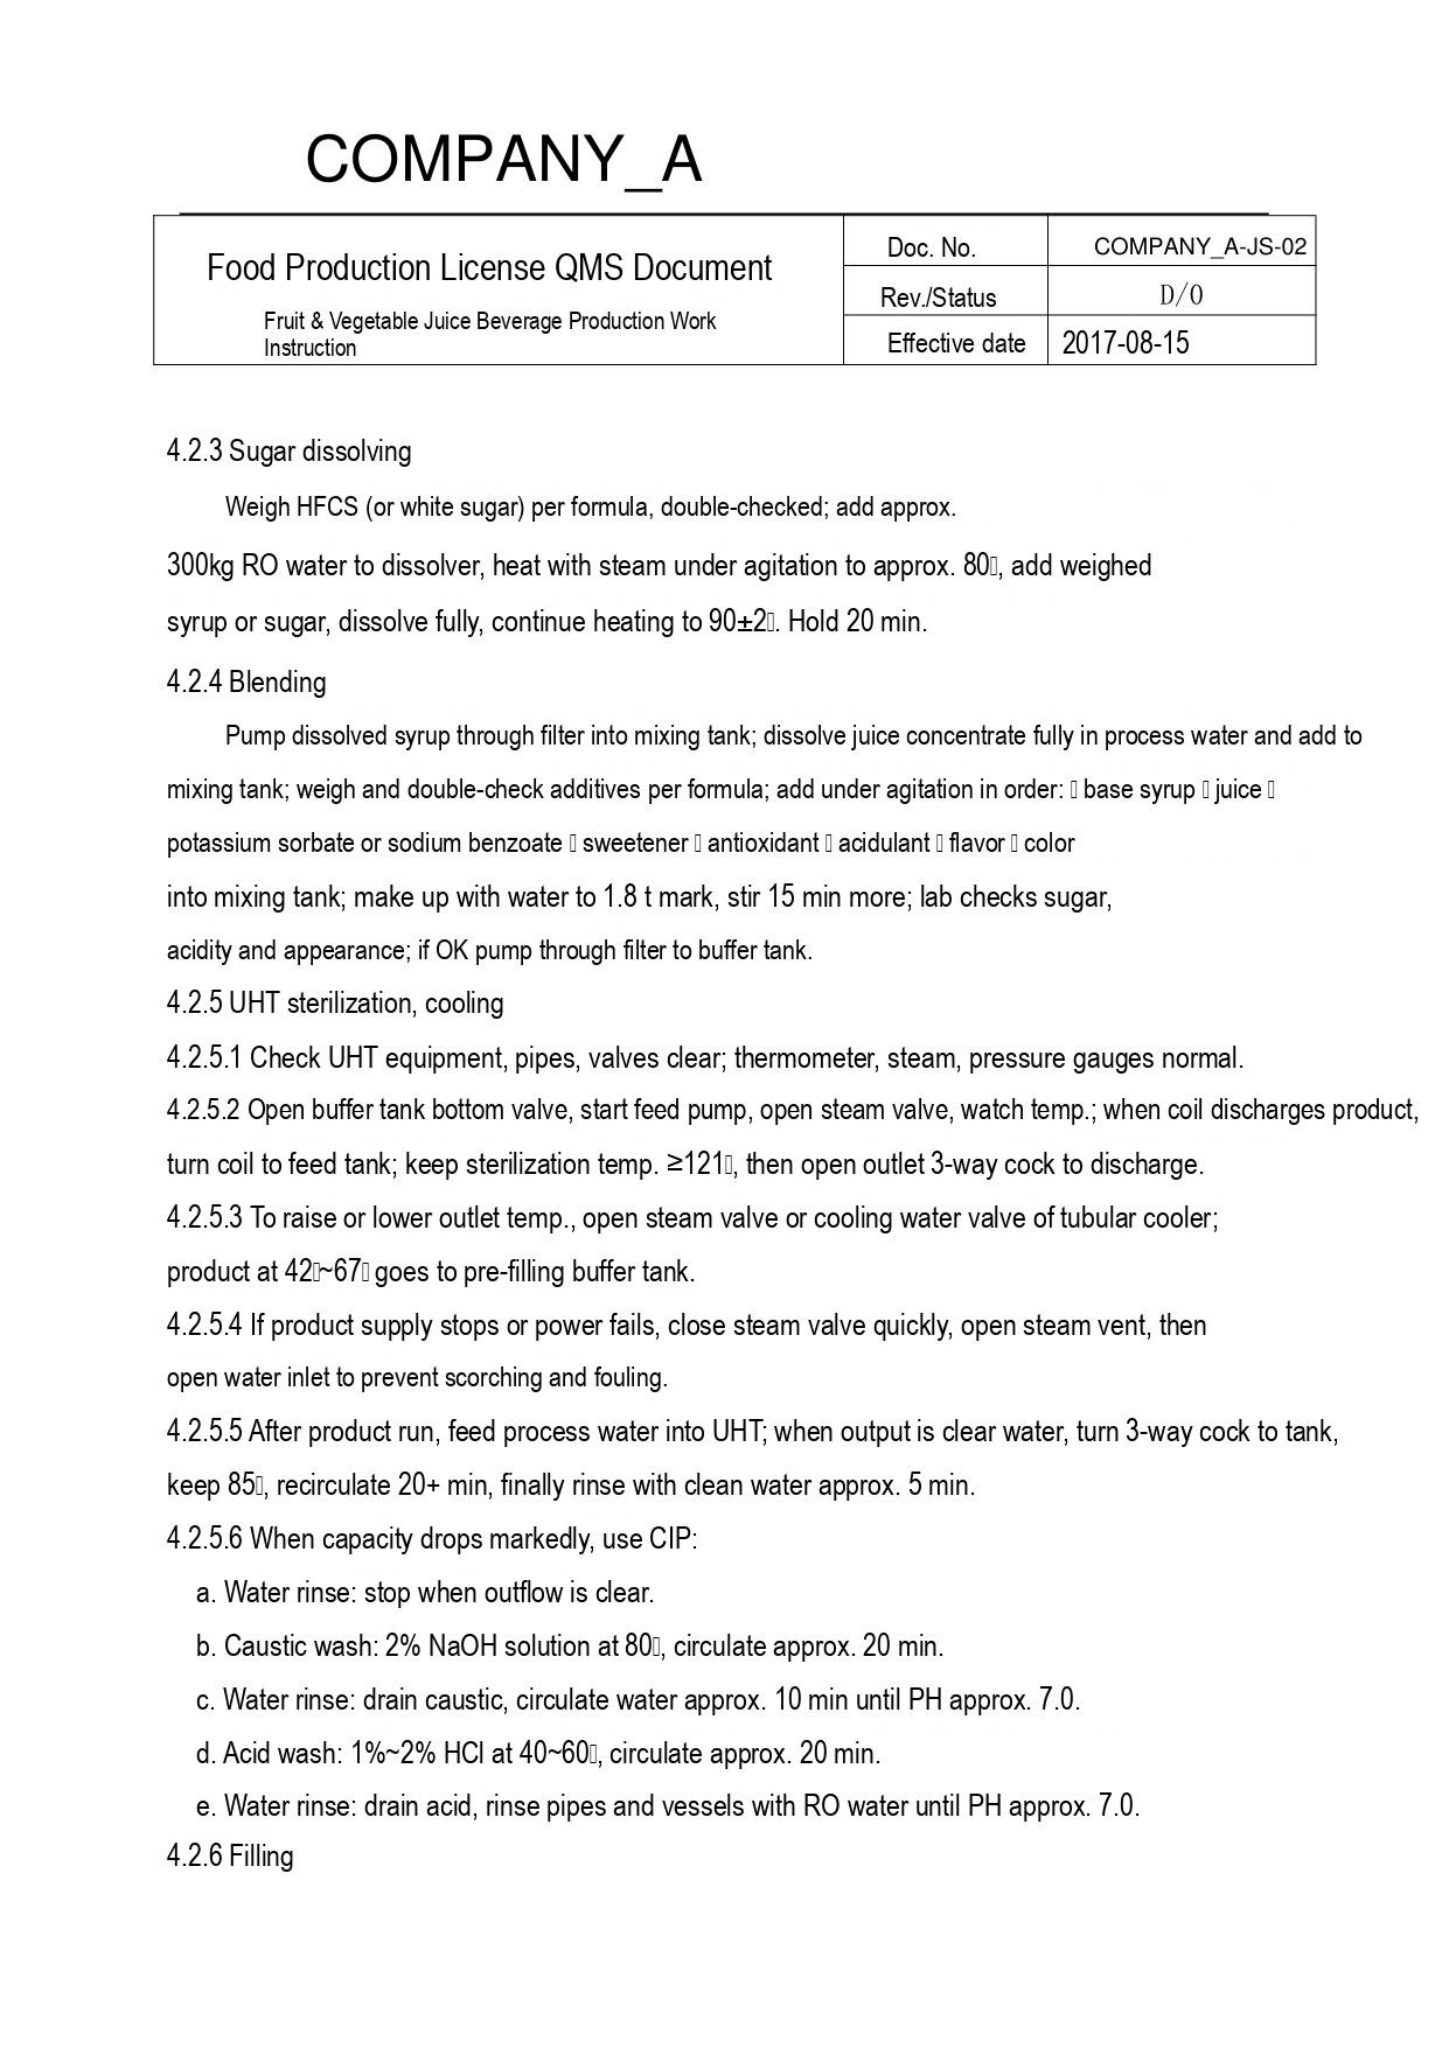COMPANY_A

| Food Production License QMS Document<br>Fruit & Vegetable Juice Beverage Production Work Instruction | Doc. No. | COMPANY_A-JS-02 |
|---|---|---|
| | Rev./Status | D/0 |
| | Effective date | 2017-08-15 |

4.2.3 Sugar dissolving

Weigh HFCS (or white sugar) per formula, double-checked; add approx. 300kg RO water to dissolver, heat with steam under agitation to approx. 80□, add weighed syrup or sugar, dissolve fully, continue heating to 90±2□. Hold 20 min.

4.2.4 Blending

Pump dissolved syrup through filter into mixing tank; dissolve juice concentrate fully in process water and add to mixing tank; weigh and double-check additives per formula; add under agitation in order: □ base syrup □ juice □ potassium sorbate or sodium benzoate □ sweetener □ antioxidant □ acidulant □ flavor □ color into mixing tank; make up with water to 1.8 t mark, stir 15 min more; lab checks sugar, acidity and appearance; if OK pump through filter to buffer tank.

4.2.5 UHT sterilization, cooling

4.2.5.1 Check UHT equipment, pipes, valves clear; thermometer, steam, pressure gauges normal.

4.2.5.2 Open buffer tank bottom valve, start feed pump, open steam valve, watch temp.; when coil discharges product, turn coil to feed tank; keep sterilization temp. ≥121□, then open outlet 3-way cock to discharge.

4.2.5.3 To raise or lower outlet temp., open steam valve or cooling water valve of tubular cooler; product at 42□~67□ goes to pre-filling buffer tank.

4.2.5.4 If product supply stops or power fails, close steam valve quickly, open steam vent, then open water inlet to prevent scorching and fouling.

4.2.5.5 After product run, feed process water into UHT; when output is clear water, turn 3-way cock to tank, keep 85□, recirculate 20+ min, finally rinse with clean water approx. 5 min.

4.2.5.6 When capacity drops markedly, use CIP:

a. Water rinse: stop when outflow is clear.

b. Caustic wash: 2% NaOH solution at 80□, circulate approx. 20 min.

c. Water rinse: drain caustic, circulate water approx. 10 min until PH approx. 7.0.

d. Acid wash: 1%~2% HCl at 40~60□, circulate approx. 20 min.

e. Water rinse: drain acid, rinse pipes and vessels with RO water until PH approx. 7.0.

4.2.6 Filling
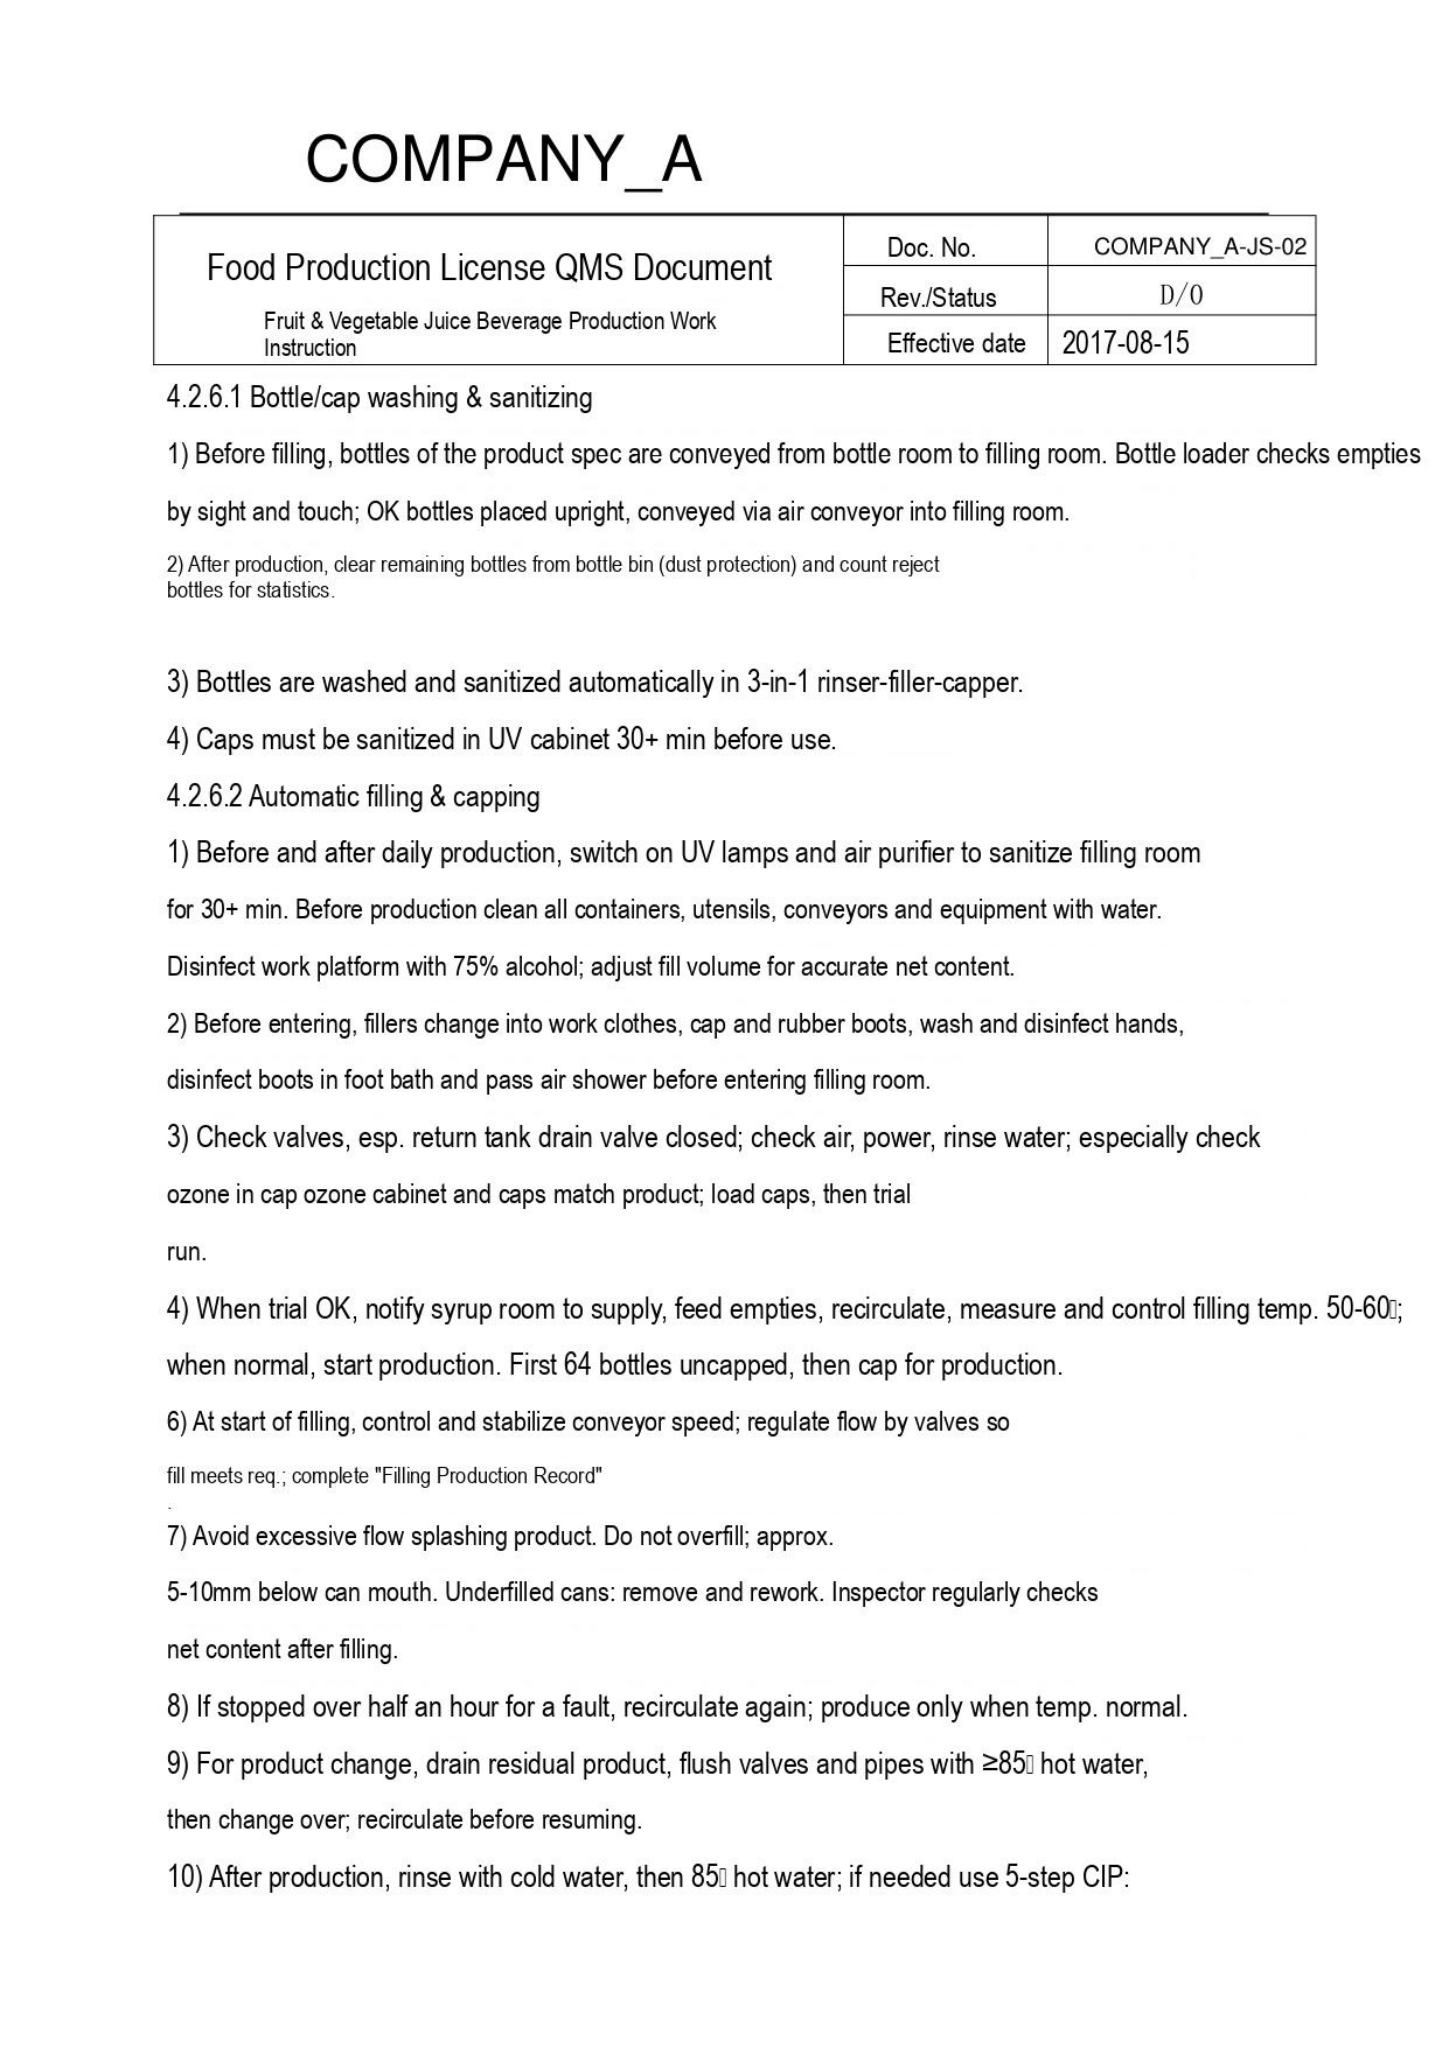COMPANY_A

| Food Production License QMS Document<br>Fruit & Vegetable Juice Beverage Production Work Instruction | Doc. No. | COMPANY_A-JS-02 |
|---|---|---|
| | Rev./Status | D/0 |
| | Effective date | 2017-08-15 |

4.2.6.1 Bottle/cap washing & sanitizing

1) Before filling, bottles of the product spec are conveyed from bottle room to filling room. Bottle loader checks empties by sight and touch; OK bottles placed upright, conveyed via air conveyor into filling room.

2) After production, clear remaining bottles from bottle bin (dust protection) and count reject bottles for statistics.

3) Bottles are washed and sanitized automatically in 3-in-1 rinser-filler-capper.

4) Caps must be sanitized in UV cabinet 30+ min before use.

4.2.6.2 Automatic filling & capping

1) Before and after daily production, switch on UV lamps and air purifier to sanitize filling room for 30+ min. Before production clean all containers, utensils, conveyors and equipment with water. Disinfect work platform with 75% alcohol; adjust fill volume for accurate net content.

2) Before entering, fillers change into work clothes, cap and rubber boots, wash and disinfect hands, disinfect boots in foot bath and pass air shower before entering filling room.

3) Check valves, esp. return tank drain valve closed; check air, power, rinse water; especially check ozone in cap ozone cabinet and caps match product; load caps, then trial run.

4) When trial OK, notify syrup room to supply, feed empties, recirculate, measure and control filling temp. 50-60; when normal, start production. First 64 bottles uncapped, then cap for production.

6) At start of filling, control and stabilize conveyor speed; regulate flow by valves so fill meets req.; complete "Filling Production Record"

7) Avoid excessive flow splashing product. Do not overfill; approx. 5-10mm below can mouth. Underfilled cans: remove and rework. Inspector regularly checks net content after filling.

8) If stopped over half an hour for a fault, recirculate again; produce only when temp. normal.

9) For product change, drain residual product, flush valves and pipes with ≥85 hot water, then change over; recirculate before resuming.

10) After production, rinse with cold water, then 85 hot water; if needed use 5-step CIP:
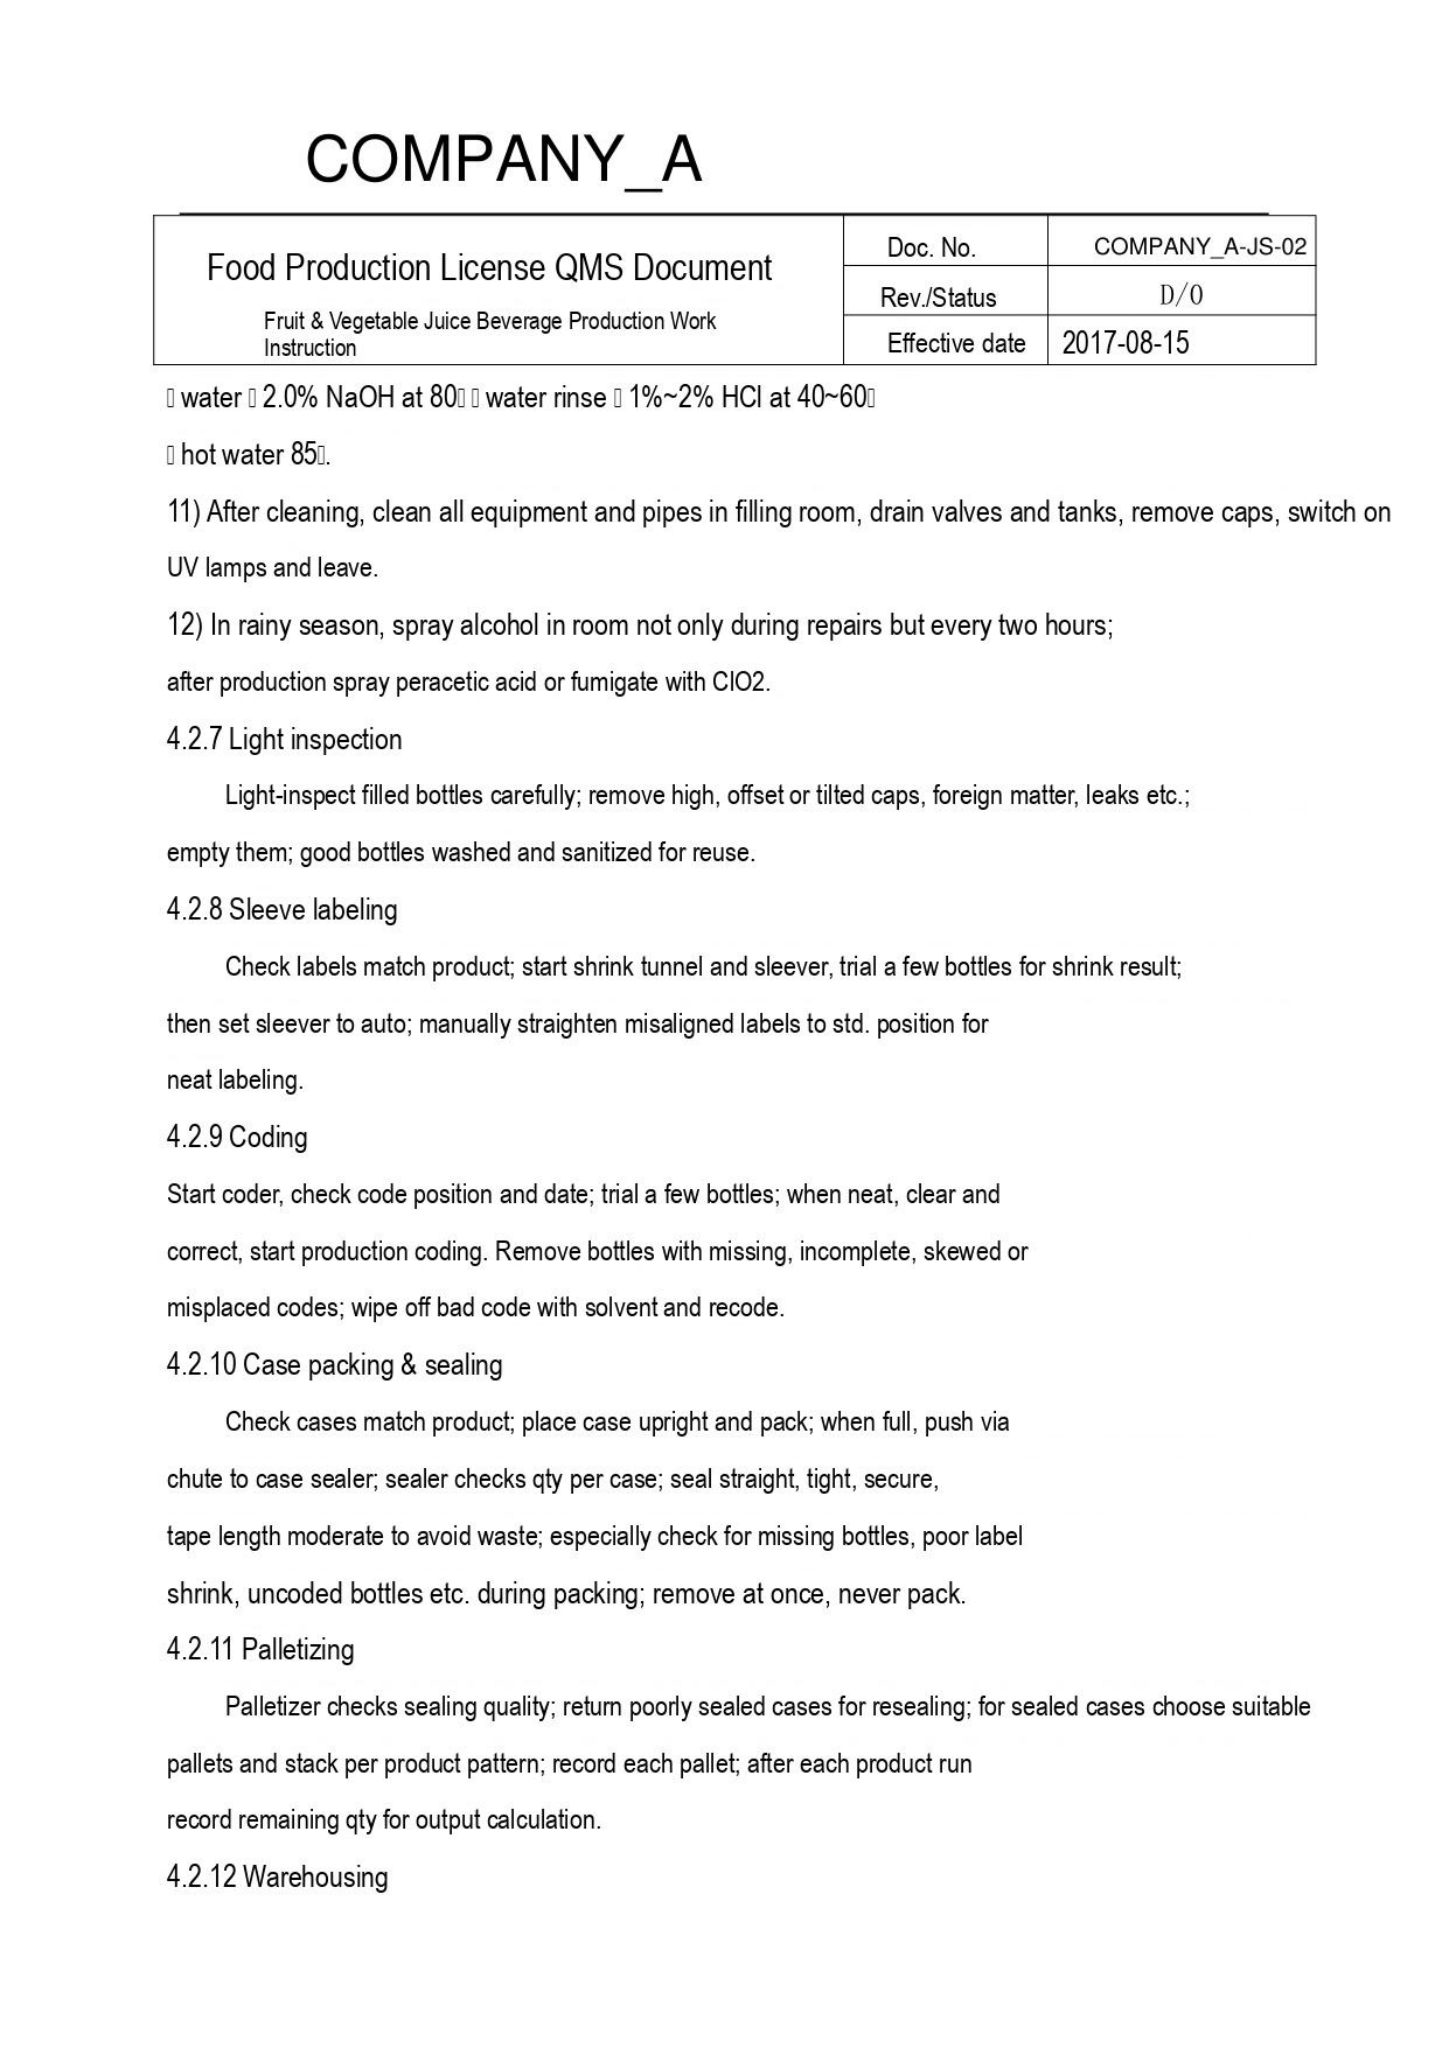COMPANY_A

| Food Production License QMS Document<br>Fruit & Vegetable Juice Beverage Production Work Instruction | Doc. No. | COMPANY_A-JS-02 |
|---|---|---|
| | Rev./Status | D/0 |
| | Effective date | 2017-08-15 |

water 2.0% NaOH at 80 water rinse 1%~2% HCl at 40~60

hot water 85.

11) After cleaning, clean all equipment and pipes in filling room, drain valves and tanks, remove caps, switch on UV lamps and leave.

12) In rainy season, spray alcohol in room not only during repairs but every two hours; after production spray peracetic acid or fumigate with ClO2.

4.2.7 Light inspection

Light-inspect filled bottles carefully; remove high, offset or tilted caps, foreign matter, leaks etc.; empty them; good bottles washed and sanitized for reuse.

4.2.8 Sleeve labeling

Check labels match product; start shrink tunnel and sleever, trial a few bottles for shrink result; then set sleever to auto; manually straighten misaligned labels to std. position for neat labeling.

4.2.9 Coding

Start coder, check code position and date; trial a few bottles; when neat, clear and correct, start production coding. Remove bottles with missing, incomplete, skewed or misplaced codes; wipe off bad code with solvent and recode.

4.2.10 Case packing & sealing

Check cases match product; place case upright and pack; when full, push via chute to case sealer; sealer checks qty per case; seal straight, tight, secure, tape length moderate to avoid waste; especially check for missing bottles, poor label shrink, uncoded bottles etc. during packing; remove at once, never pack.

4.2.11 Palletizing

Palletizer checks sealing quality; return poorly sealed cases for resealing; for sealed cases choose suitable pallets and stack per product pattern; record each pallet; after each product run record remaining qty for output calculation.

4.2.12 Warehousing
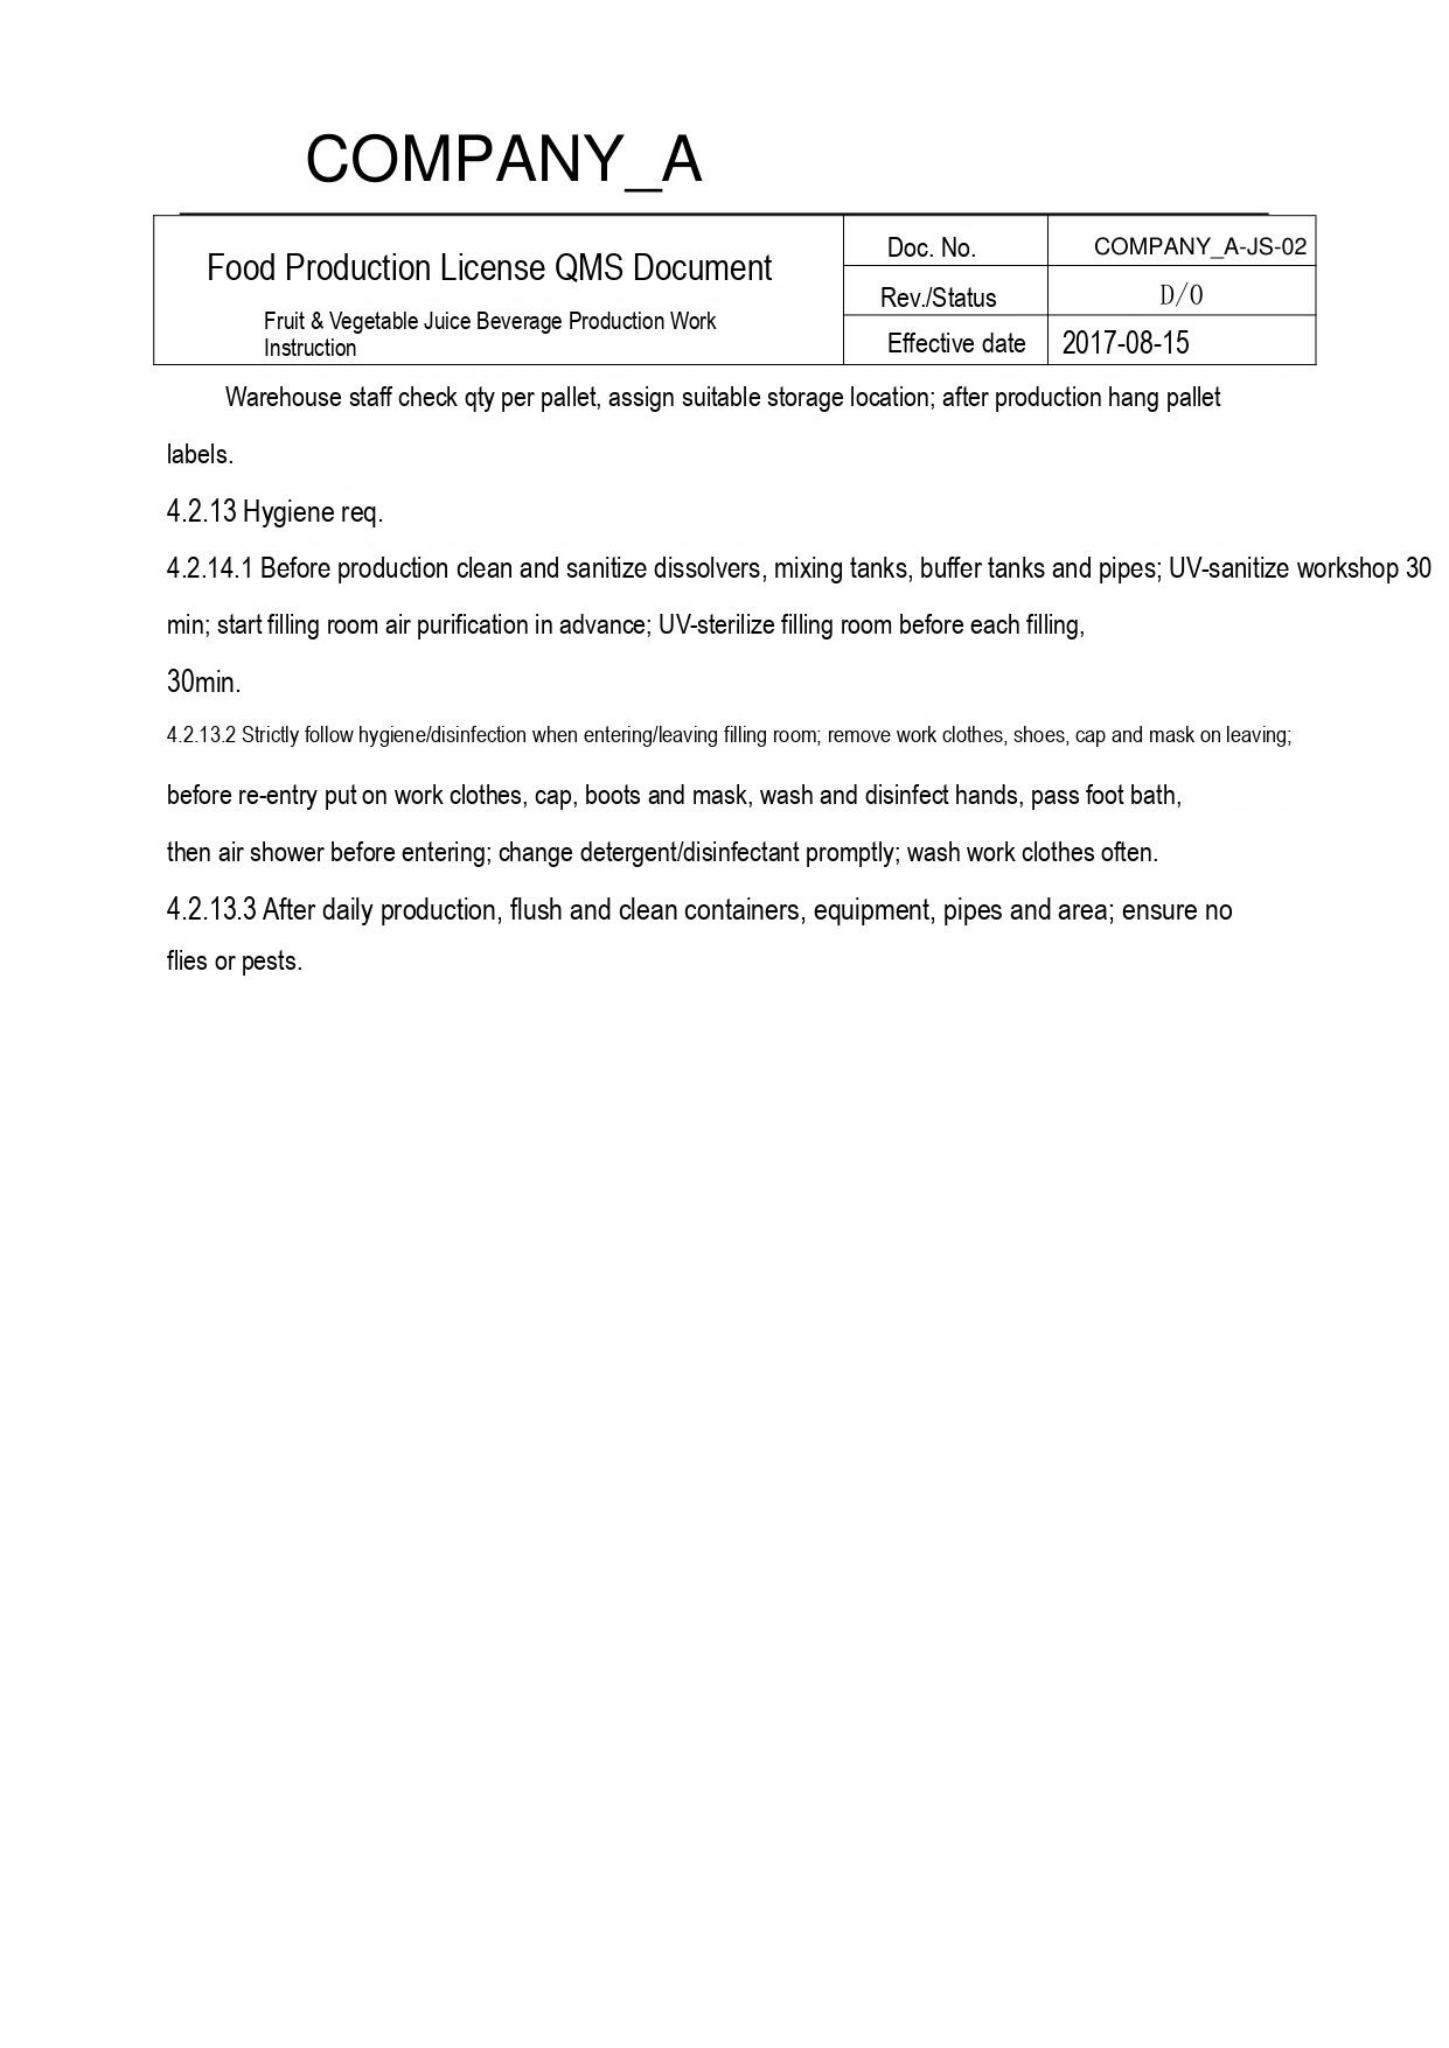COMPANY_A

| Food Production License QMS Document<br>Fruit & Vegetable Juice Beverage Production Work Instruction | Doc. No. | COMPANY_A-JS-02 |
|---|---|---|
| | Rev./Status | D/0 |
| | Effective date | 2017-08-15 |

Warehouse staff check qty per pallet, assign suitable storage location; after production hang pallet labels.

4.2.13 Hygiene req.

4.2.14.1 Before production clean and sanitize dissolvers, mixing tanks, buffer tanks and pipes; UV-sanitize workshop 30 min; start filling room air purification in advance; UV-sterilize filling room before each filling, 30min.

4.2.13.2 Strictly follow hygiene/disinfection when entering/leaving filling room; remove work clothes, shoes, cap and mask on leaving; before re-entry put on work clothes, cap, boots and mask, wash and disinfect hands, pass foot bath, then air shower before entering; change detergent/disinfectant promptly; wash work clothes often.

4.2.13.3 After daily production, flush and clean containers, equipment, pipes and area; ensure no flies or pests.
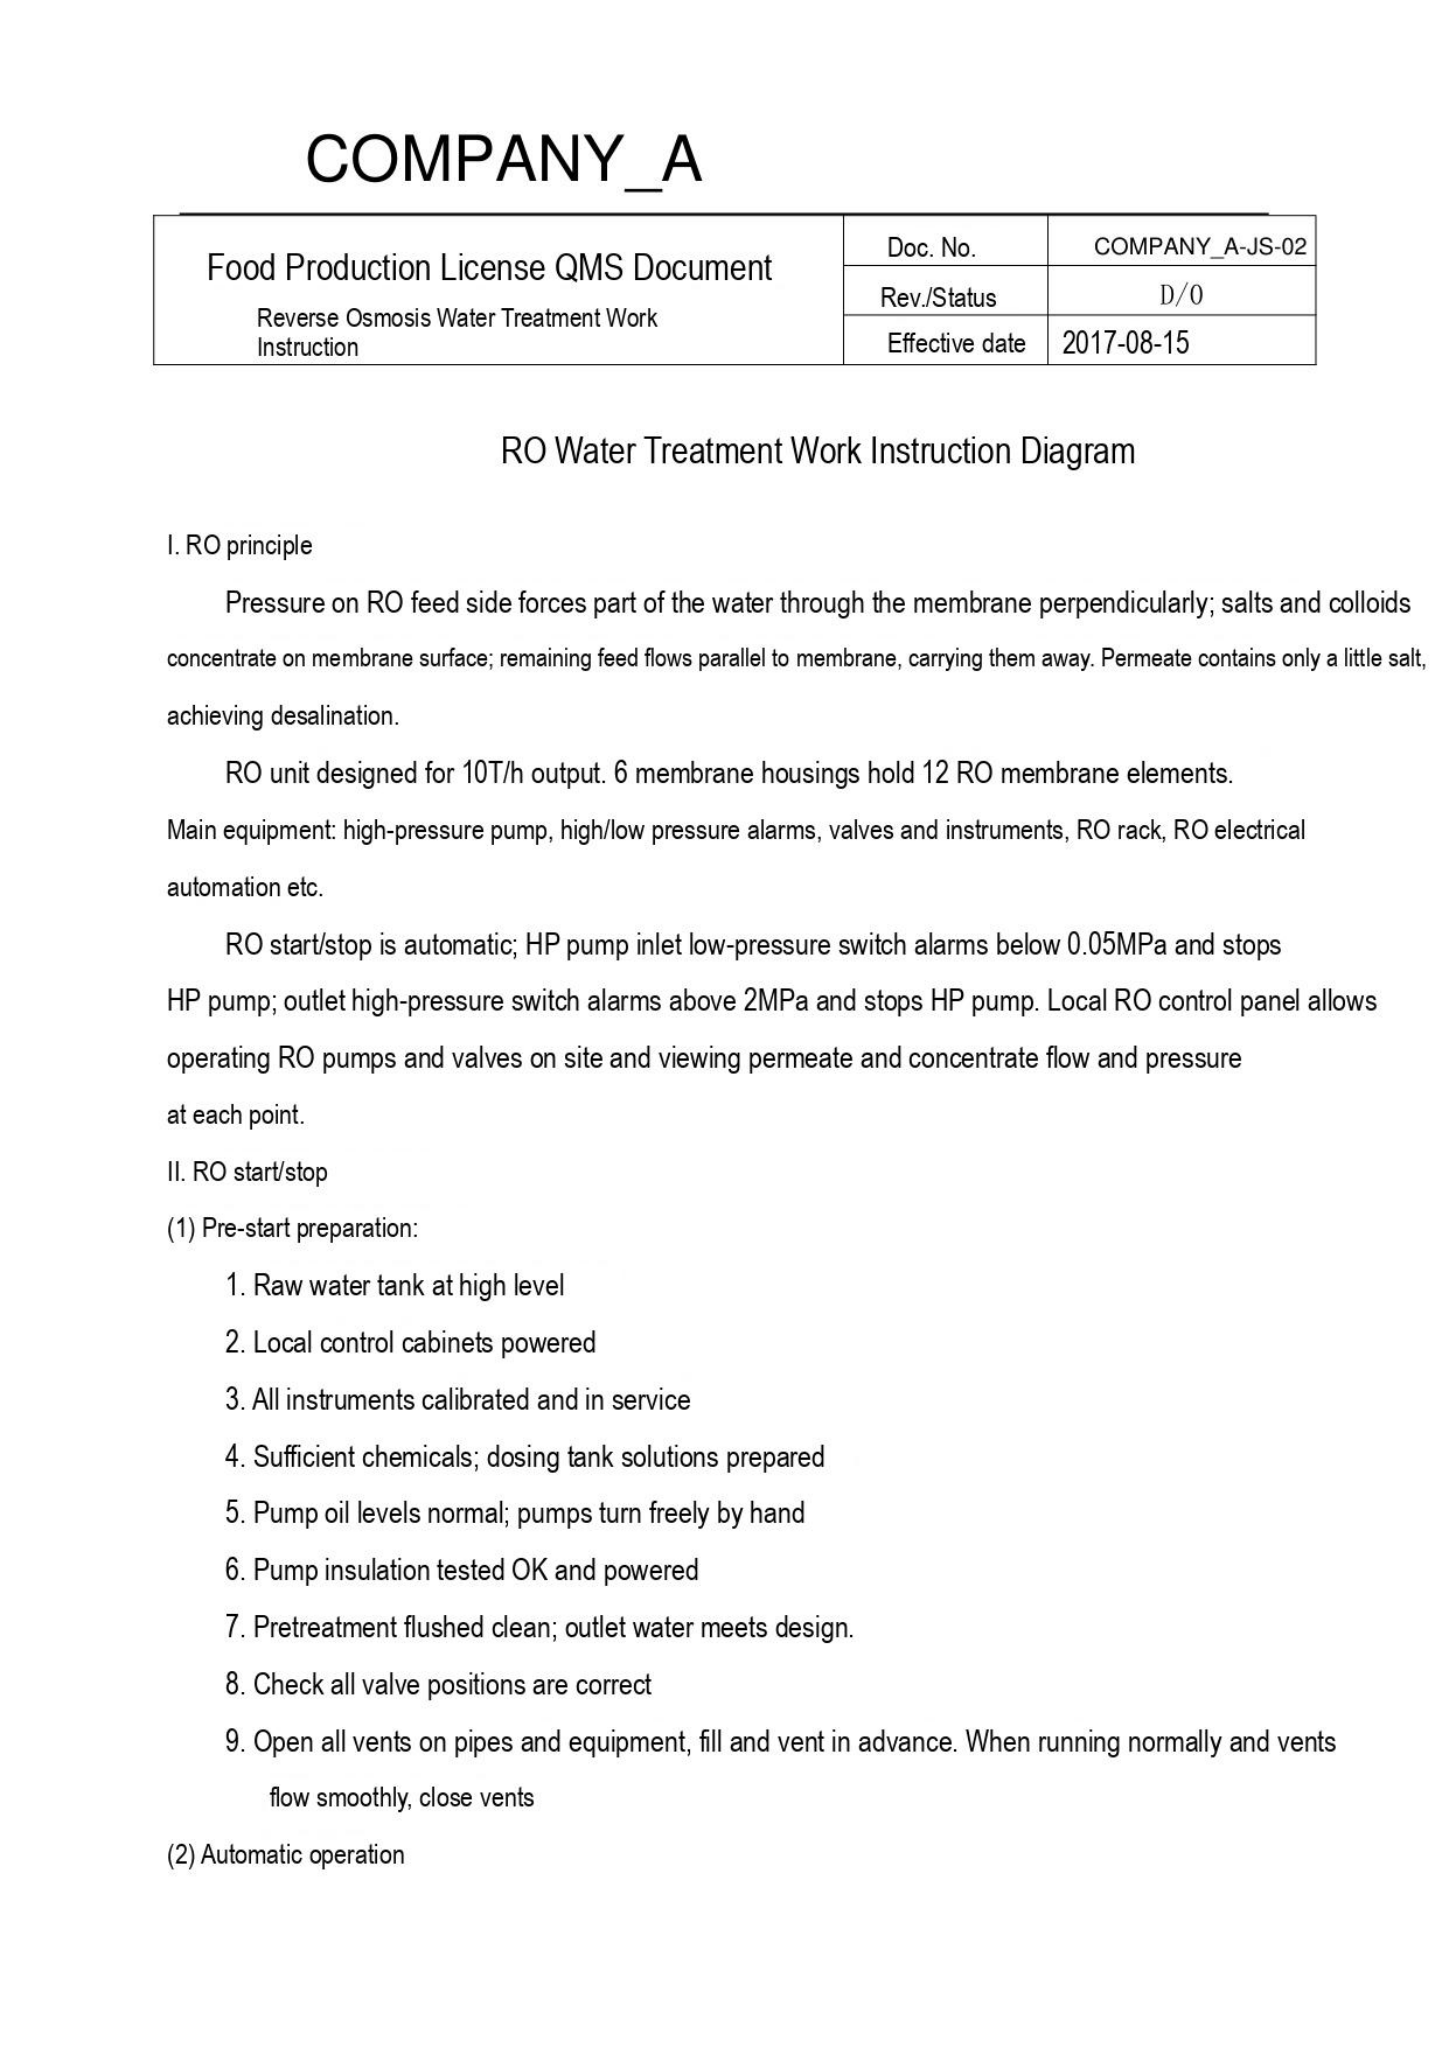COMPANY_A

| Food Production License QMS Document<br>Reverse Osmosis Water Treatment Work Instruction | Doc. No. | COMPANY_A-JS-02 |
|---|---|---|
| | Rev./Status | D/0 |
| | Effective date | 2017-08-15 |

RO Water Treatment Work Instruction Diagram

I. RO principle

Pressure on RO feed side forces part of the water through the membrane perpendicularly; salts and colloids concentrate on membrane surface; remaining feed flows parallel to membrane, carrying them away. Permeate contains only a little salt, achieving desalination.

RO unit designed for 10T/h output. 6 membrane housings hold 12 RO membrane elements. Main equipment: high-pressure pump, high/low pressure alarms, valves and instruments, RO rack, RO electrical automation etc.

RO start/stop is automatic; HP pump inlet low-pressure switch alarms below 0.05MPa and stops HP pump; outlet high-pressure switch alarms above 2MPa and stops HP pump. Local RO control panel allows operating RO pumps and valves on site and viewing permeate and concentrate flow and pressure at each point.

II. RO start/stop

(1) Pre-start preparation:

1. Raw water tank at high level
2. Local control cabinets powered
3. All instruments calibrated and in service
4. Sufficient chemicals; dosing tank solutions prepared
5. Pump oil levels normal; pumps turn freely by hand
6. Pump insulation tested OK and powered
7. Pretreatment flushed clean; outlet water meets design.
8. Check all valve positions are correct
9. Open all vents on pipes and equipment, fill and vent in advance. When running normally and vents flow smoothly, close vents

(2) Automatic operation
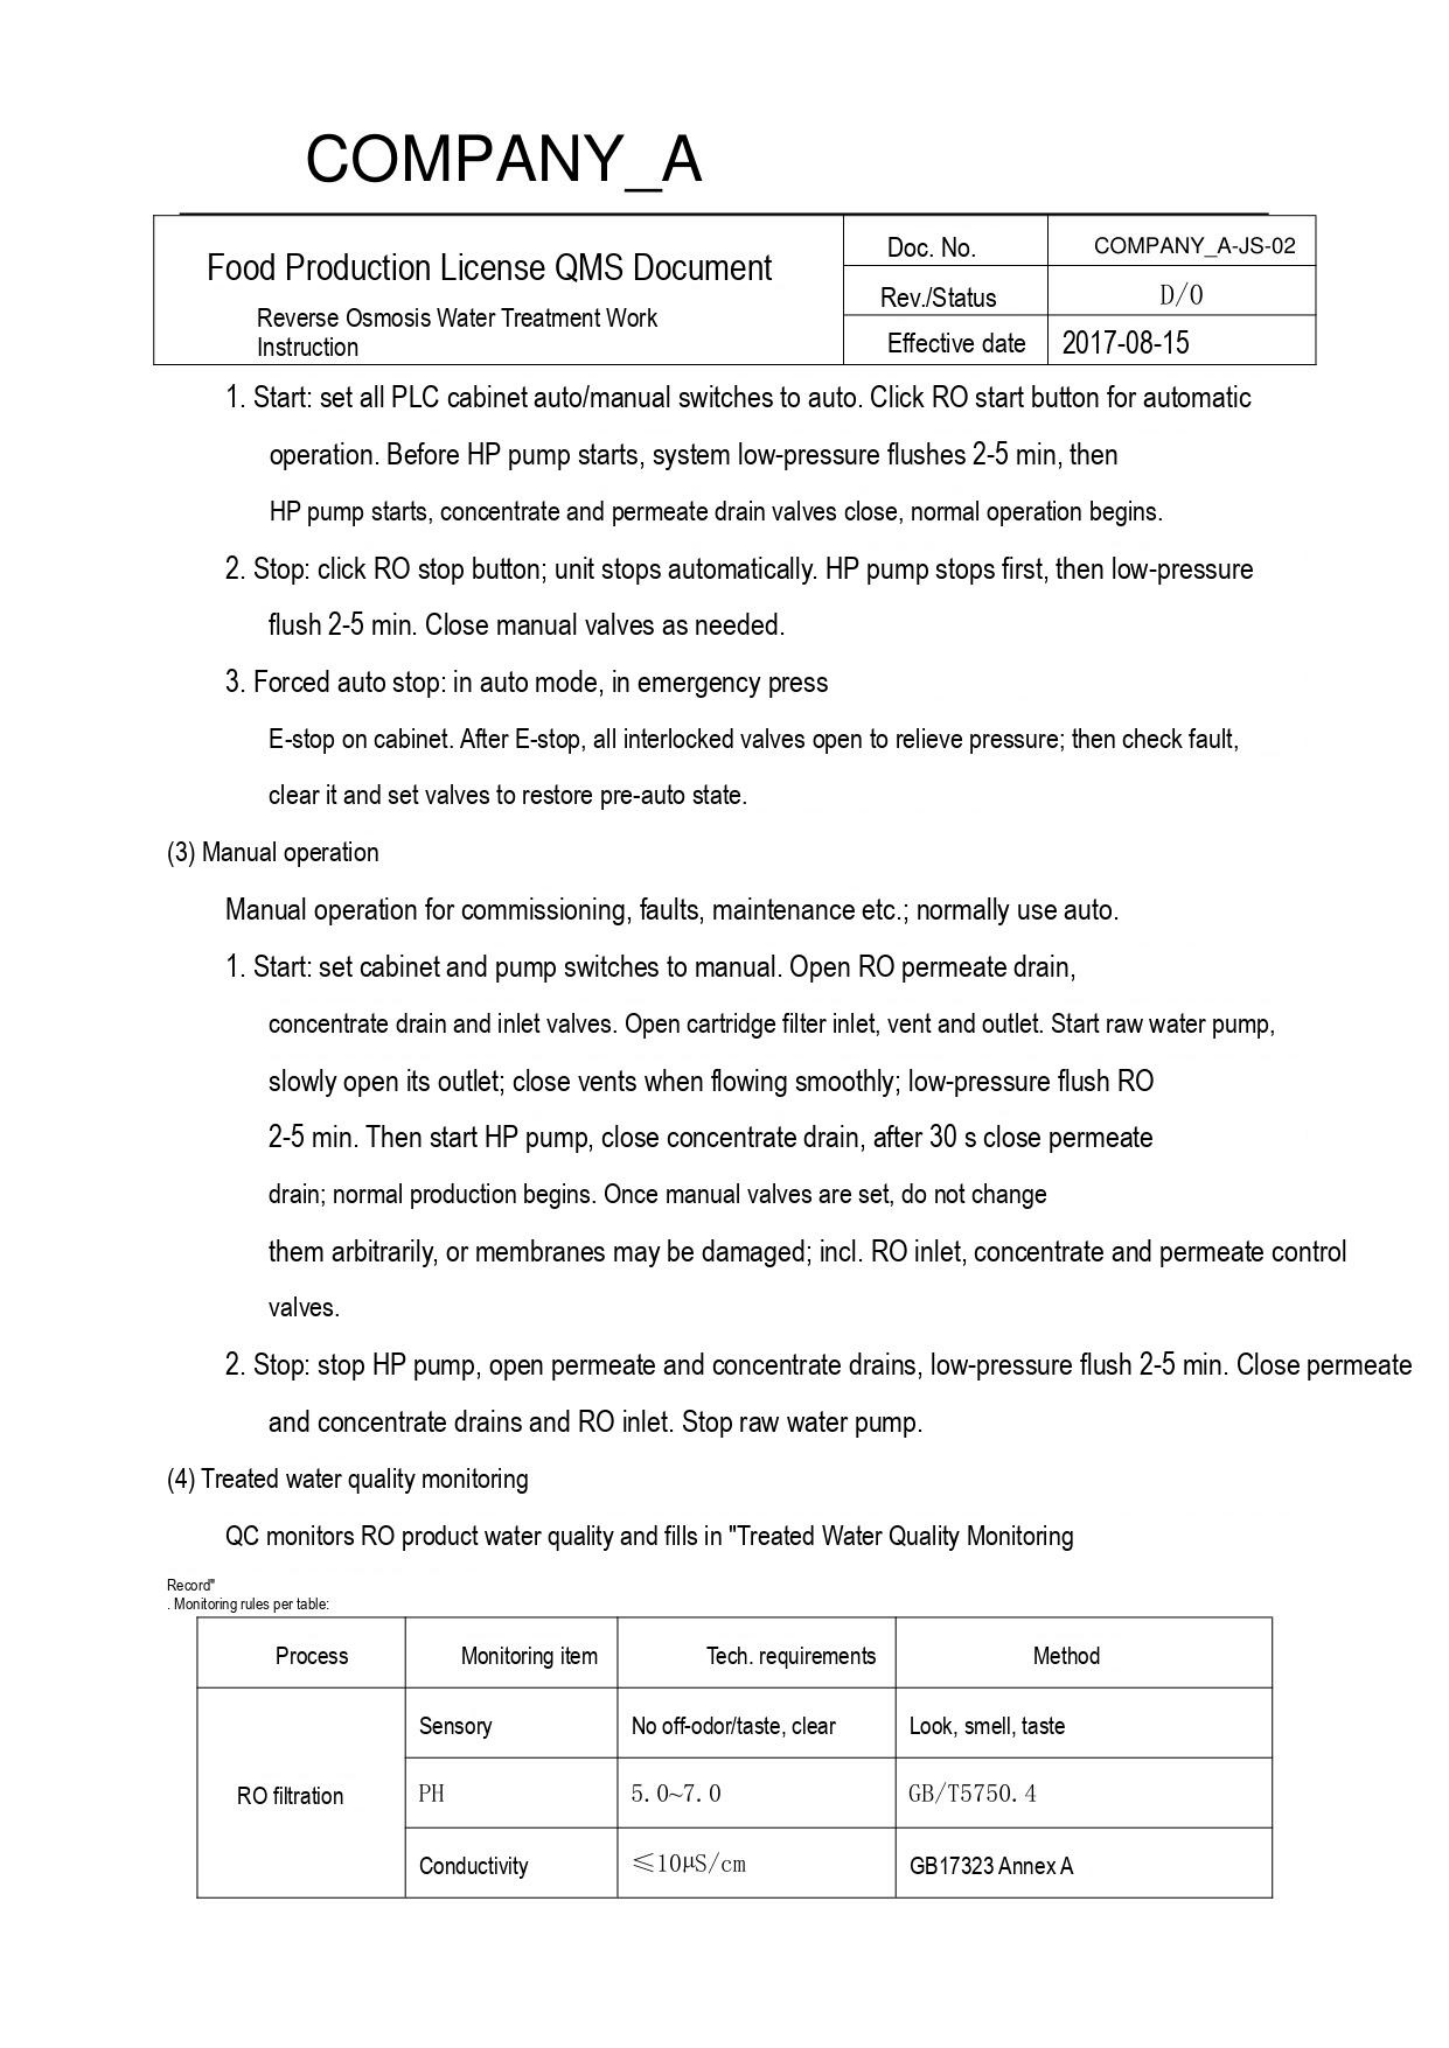COMPANY_A

| Food Production License QMS Document<br>Reverse Osmosis Water Treatment Work Instruction | Doc. No. | COMPANY_A-JS-02 |
|---|---|---|
| | Rev./Status | D/0 |
| | Effective date | 2017-08-15 |

1. Start: set all PLC cabinet auto/manual switches to auto. Click RO start button for automatic operation. Before HP pump starts, system low-pressure flushes 2-5 min, then HP pump starts, concentrate and permeate drain valves close, normal operation begins.

2. Stop: click RO stop button; unit stops automatically. HP pump stops first, then low-pressure flush 2-5 min. Close manual valves as needed.

3. Forced auto stop: in auto mode, in emergency press E-stop on cabinet. After E-stop, all interlocked valves open to relieve pressure; then check fault, clear it and set valves to restore pre-auto state.

(3) Manual operation

Manual operation for commissioning, faults, maintenance etc.; normally use auto.

1. Start: set cabinet and pump switches to manual. Open RO permeate drain, concentrate drain and inlet valves. Open cartridge filter inlet, vent and outlet. Start raw water pump, slowly open its outlet; close vents when flowing smoothly; low-pressure flush RO 2-5 min. Then start HP pump, close concentrate drain, after 30 s close permeate drain; normal production begins. Once manual valves are set, do not change them arbitrarily, or membranes may be damaged; incl. RO inlet, concentrate and permeate control valves.

2. Stop: stop HP pump, open permeate and concentrate drains, low-pressure flush 2-5 min. Close permeate and concentrate drains and RO inlet. Stop raw water pump.

(4) Treated water quality monitoring

QC monitors RO product water quality and fills in "Treated Water Quality Monitoring Record"
. Monitoring rules per table:

| Process | Monitoring item | Tech. requirements | Method |
|---|---|---|---|
| RO filtration | Sensory | No off-odor/taste, clear | Look, smell, taste |
| | PH | 5.0~7.0 | GB/T5750.4 |
| | Conductivity | ≤10μS/cm | GB17323 Annex A |